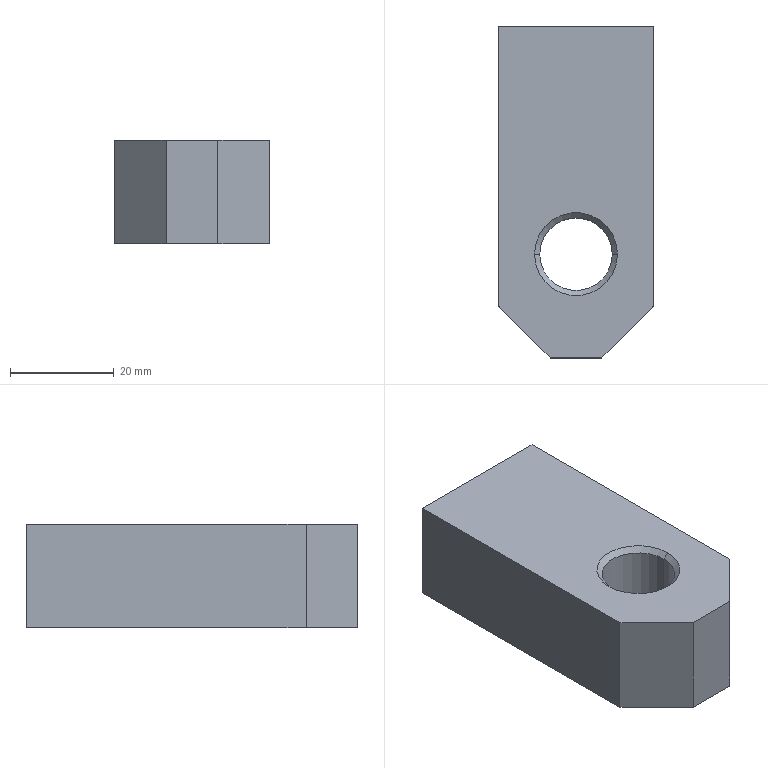Part | STEP file | BCC3 H12_4B | 1 solid | 18 faces | box 30 x 64 x 20 mm | volume 31837 mm3 | plane 8 | cone 6 | cylinder 4 | commonest cylinder face diameters 8.5 x2 14 x2
STEP:
#1=CARTESIAN_POINT('',(0.,0.,0.));
#2=DIRECTION('',(0.,0.,1.));
#3=DIRECTION('',(1.,0.,0.));
#4=AXIS2_PLACEMENT_3D('',#1,#2,#3);
#5=CARTESIAN_POINT('',(7.,-12.,9.));
#6=VERTEX_POINT('',#5);
#7=CARTESIAN_POINT('',(8.,-12.,10.));
#8=VERTEX_POINT('',#7);
#9=CARTESIAN_POINT('',(7.,-12.,9.));
#10=DIRECTION('',(0.7071,0.,0.7071));
#11=VECTOR('',#10,1.);
#12=LINE('',#9,#11);
#13=CARTESIAN_POINT('',(0.,-12.,9.));
#14=DIRECTION('',(0.,0.,1.));
#15=DIRECTION('',(1.,0.,0.));
#16=AXIS2_PLACEMENT_3D('',#13,#14,#15);
#17=CONICAL_SURFACE('',#16,7.,0.7854);
#18=CARTESIAN_POINT('',(6.283,0.));
#19=DIRECTION('',(0.,1.));
#20=VECTOR('',#19,1.);
#21=LINE('',#18,#20);
#22=(GEOMETRIC_REPRESENTATION_CONTEXT(2)PARAMETRIC_REPRESENTATION_CONTEXT()REPRESENTATION_CONTEXT('',''));
#23=DEFINITIONAL_REPRESENTATION('',(#21),#22);
#24=PCURVE('',#17,#23);
#25=CARTESIAN_POINT('',(0.,-12.,9.));
#26=DIRECTION('',(0.,0.,1.));
#27=DIRECTION('',(1.,0.,0.));
#28=AXIS2_PLACEMENT_3D('',#25,#26,#27);
#29=CONICAL_SURFACE('',#28,7.,0.7854);
#30=CARTESIAN_POINT('',(0.,0.));
#31=DIRECTION('',(0.,1.));
#32=VECTOR('',#31,1.);
#33=LINE('',#30,#32);
#34=(GEOMETRIC_REPRESENTATION_CONTEXT(2)PARAMETRIC_REPRESENTATION_CONTEXT()REPRESENTATION_CONTEXT('',''));
#35=DEFINITIONAL_REPRESENTATION('',(#33),#34);
#36=PCURVE('',#29,#35);
#37=SURFACE_CURVE('',#12,(#24,#36),.PCURVE_S1.);
#38=EDGE_CURVE('',#6,#8,#37,.T.);
#39=ORIENTED_EDGE('',*,*,#38,.T.);
#40=CARTESIAN_POINT('',(-8.,-12.,10.));
#41=VERTEX_POINT('',#40);
#42=CARTESIAN_POINT('',(0.,-12.,10.));
#43=DIRECTION('',(0.,0.,-1.));
#44=DIRECTION('',(1.,0.,0.));
#45=AXIS2_PLACEMENT_3D('',#42,#43,#44);
#46=CIRCLE('',#45,8.);
#47=CARTESIAN_POINT('',(6.283,1.));
#48=DIRECTION('',(-1.,0.));
#49=VECTOR('',#48,1.);
#50=LINE('',#47,#49);
#51=(GEOMETRIC_REPRESENTATION_CONTEXT(2)PARAMETRIC_REPRESENTATION_CONTEXT()REPRESENTATION_CONTEXT('',''));
#52=DEFINITIONAL_REPRESENTATION('',(#50),#51);
#53=PCURVE('',#17,#52);
#54=CARTESIAN_POINT('',(0.,0.,10.));
#55=DIRECTION('',(0.,0.,1.));
#56=DIRECTION('',(1.,0.,0.));
#57=AXIS2_PLACEMENT_3D('',#54,#55,#56);
#58=PLANE('',#57);
#59=CARTESIAN_POINT('',(8.,-12.));
#60=CARTESIAN_POINT('',(8.,-25.856));
#61=CARTESIAN_POINT('',(-4.,-18.928));
#62=CARTESIAN_POINT('',(-16.,-12.));
#63=CARTESIAN_POINT('',(-4.,-5.072));
#64=CARTESIAN_POINT('',(8.,1.856));
#65=CARTESIAN_POINT('',(8.,-12.));
#66=(BOUNDED_CURVE()B_SPLINE_CURVE(2,(#59,#60,#61,#62,#63,#64,#65),.UNSPECIFIED.,.T.,.F.)B_SPLINE_CURVE_WITH_KNOTS((1,2,2,2,2,1),(-2.094,0.,2.094,4.189,6.283,8.378),.UNSPECIFIED.)CURVE()GEOMETRIC_REPRESENTATION_ITEM()RATIONAL_B_SPLINE_CURVE((1.,0.5,1.,0.5,1.,0.5,1.))REPRESENTATION_ITEM(''));
#67=(GEOMETRIC_REPRESENTATION_CONTEXT(2)PARAMETRIC_REPRESENTATION_CONTEXT()REPRESENTATION_CONTEXT('',''));
#68=DEFINITIONAL_REPRESENTATION('',(#66),#67);
#69=PCURVE('',#58,#68);
#70=SURFACE_CURVE('',#46,(#53,#69),.PCURVE_S1.);
#71=EDGE_CURVE('',#8,#41,#70,.T.);
#72=ORIENTED_EDGE('',*,*,#71,.T.);
#73=CARTESIAN_POINT('',(-7.,-12.,9.));
#74=VERTEX_POINT('',#73);
#75=CARTESIAN_POINT('',(-7.,-12.,9.));
#76=DIRECTION('',(-0.7071,0.,0.7071));
#77=VECTOR('',#76,1.);
#78=LINE('',#75,#77);
#79=CARTESIAN_POINT('',(3.142,0.));
#80=DIRECTION('',(0.,1.));
#81=VECTOR('',#80,1.);
#82=LINE('',#79,#81);
#83=(GEOMETRIC_REPRESENTATION_CONTEXT(2)PARAMETRIC_REPRESENTATION_CONTEXT()REPRESENTATION_CONTEXT('',''));
#84=DEFINITIONAL_REPRESENTATION('',(#82),#83);
#85=PCURVE('',#17,#84);
#86=CARTESIAN_POINT('',(3.142,0.));
#87=DIRECTION('',(0.,1.));
#88=VECTOR('',#87,1.);
#89=LINE('',#86,#88);
#90=(GEOMETRIC_REPRESENTATION_CONTEXT(2)PARAMETRIC_REPRESENTATION_CONTEXT()REPRESENTATION_CONTEXT('',''));
#91=DEFINITIONAL_REPRESENTATION('',(#89),#90);
#92=PCURVE('',#29,#91);
#93=SURFACE_CURVE('',#78,(#85,#92),.PCURVE_S1.);
#94=EDGE_CURVE('',#74,#41,#93,.T.);
#95=ORIENTED_EDGE('',*,*,#94,.F.);
#96=CARTESIAN_POINT('',(0.,-12.,9.));
#97=DIRECTION('',(0.,0.,1.));
#98=DIRECTION('',(1.,0.,0.));
#99=AXIS2_PLACEMENT_3D('',#96,#97,#98);
#100=CIRCLE('',#99,7.);
#101=CARTESIAN_POINT('',(0.,0.));
#102=DIRECTION('',(1.,0.));
#103=VECTOR('',#102,1.);
#104=LINE('',#101,#103);
#105=(GEOMETRIC_REPRESENTATION_CONTEXT(2)PARAMETRIC_REPRESENTATION_CONTEXT()REPRESENTATION_CONTEXT('',''));
#106=DEFINITIONAL_REPRESENTATION('',(#104),#105);
#107=PCURVE('',#17,#106);
#108=CARTESIAN_POINT('',(0.,-12.,10.));
#109=DIRECTION('',(0.,0.,-1.));
#110=DIRECTION('',(-1.,0.,0.));
#111=AXIS2_PLACEMENT_3D('',#108,#109,#110);
#112=CYLINDRICAL_SURFACE('',#111,7.);
#113=CARTESIAN_POINT('',(9.425,1.));
#114=DIRECTION('',(-1.,0.));
#115=VECTOR('',#114,1.);
#116=LINE('',#113,#115);
#117=(GEOMETRIC_REPRESENTATION_CONTEXT(2)PARAMETRIC_REPRESENTATION_CONTEXT()REPRESENTATION_CONTEXT('',''));
#118=DEFINITIONAL_REPRESENTATION('',(#116),#117);
#119=PCURVE('',#112,#118);
#120=SURFACE_CURVE('',#100,(#107,#119),.PCURVE_S1.);
#121=EDGE_CURVE('',#74,#6,#120,.T.);
#122=ORIENTED_EDGE('',*,*,#121,.T.);
#123=EDGE_LOOP('',(#39,#72,#95,#122));
#124=FACE_BOUND('',#123,.F.);
#125=ADVANCED_FACE('',(#124),#17,.F.);
#126=CARTESIAN_POINT('',(-7.,-12.,-9.));
#127=VERTEX_POINT('',#126);
#128=CARTESIAN_POINT('',(-8.,-12.,-10.));
#129=VERTEX_POINT('',#128);
#130=CARTESIAN_POINT('',(-8.,-12.,-10.));
#131=DIRECTION('',(-0.7071,0.,-0.7071));
#132=VECTOR('',#131,1.);
#133=LINE('',#130,#132);
#134=CARTESIAN_POINT('',(0.,-12.,-10.));
#135=DIRECTION('',(0.,0.,-1.));
#136=DIRECTION('',(-1.,0.,0.));
#137=AXIS2_PLACEMENT_3D('',#134,#135,#136);
#138=CONICAL_SURFACE('',#137,8.,0.7854);
#139=CARTESIAN_POINT('',(6.283,0.));
#140=DIRECTION('',(0.,1.));
#141=VECTOR('',#140,1.);
#142=LINE('',#139,#141);
#143=(GEOMETRIC_REPRESENTATION_CONTEXT(2)PARAMETRIC_REPRESENTATION_CONTEXT()REPRESENTATION_CONTEXT('',''));
#144=DEFINITIONAL_REPRESENTATION('',(#142),#143);
#145=PCURVE('',#138,#144);
#146=CARTESIAN_POINT('',(0.,-12.,-10.));
#147=DIRECTION('',(0.,0.,-1.));
#148=DIRECTION('',(-1.,0.,0.));
#149=AXIS2_PLACEMENT_3D('',#146,#147,#148);
#150=CONICAL_SURFACE('',#149,8.,0.7854);
#151=CARTESIAN_POINT('',(0.,0.));
#152=DIRECTION('',(0.,1.));
#153=VECTOR('',#152,1.);
#154=LINE('',#151,#153);
#155=(GEOMETRIC_REPRESENTATION_CONTEXT(2)PARAMETRIC_REPRESENTATION_CONTEXT()REPRESENTATION_CONTEXT('',''));
#156=DEFINITIONAL_REPRESENTATION('',(#154),#155);
#157=PCURVE('',#150,#156);
#158=SURFACE_CURVE('',#133,(#145,#157),.PCURVE_S1.);
#159=EDGE_CURVE('',#127,#129,#158,.T.);
#160=ORIENTED_EDGE('',*,*,#159,.T.);
#161=CARTESIAN_POINT('',(8.,-12.,-10.));
#162=VERTEX_POINT('',#161);
#163=CARTESIAN_POINT('',(0.,-12.,-10.));
#164=DIRECTION('',(0.,0.,1.));
#165=DIRECTION('',(1.,0.,0.));
#166=AXIS2_PLACEMENT_3D('',#163,#164,#165);
#167=CIRCLE('',#166,8.);
#168=CARTESIAN_POINT('',(9.425,0.));
#169=DIRECTION('',(-1.,0.));
#170=VECTOR('',#169,1.);
#171=LINE('',#168,#170);
#172=(GEOMETRIC_REPRESENTATION_CONTEXT(2)PARAMETRIC_REPRESENTATION_CONTEXT()REPRESENTATION_CONTEXT('',''));
#173=DEFINITIONAL_REPRESENTATION('',(#171),#172);
#174=PCURVE('',#138,#173);
#175=CARTESIAN_POINT('',(0.,0.,-10.));
#176=DIRECTION('',(0.,0.,1.));
#177=DIRECTION('',(1.,0.,0.));
#178=AXIS2_PLACEMENT_3D('',#175,#176,#177);
#179=PLANE('',#178);
#180=CARTESIAN_POINT('',(0.,-12.));
#181=DIRECTION('',(1.,0.));
#182=AXIS2_PLACEMENT_2D('',#180,#181);
#183=CIRCLE('',#182,8.);
#184=(GEOMETRIC_REPRESENTATION_CONTEXT(2)PARAMETRIC_REPRESENTATION_CONTEXT()REPRESENTATION_CONTEXT('',''));
#185=DEFINITIONAL_REPRESENTATION('',(#183),#184);
#186=PCURVE('',#179,#185);
#187=SURFACE_CURVE('',#167,(#174,#186),.PCURVE_S1.);
#188=EDGE_CURVE('',#129,#162,#187,.T.);
#189=ORIENTED_EDGE('',*,*,#188,.T.);
#190=CARTESIAN_POINT('',(7.,-12.,-9.));
#191=VERTEX_POINT('',#190);
#192=CARTESIAN_POINT('',(8.,-12.,-10.));
#193=DIRECTION('',(0.7071,0.,-0.7071));
#194=VECTOR('',#193,1.);
#195=LINE('',#192,#194);
#196=CARTESIAN_POINT('',(3.142,0.));
#197=DIRECTION('',(0.,1.));
#198=VECTOR('',#197,1.);
#199=LINE('',#196,#198);
#200=(GEOMETRIC_REPRESENTATION_CONTEXT(2)PARAMETRIC_REPRESENTATION_CONTEXT()REPRESENTATION_CONTEXT('',''));
#201=DEFINITIONAL_REPRESENTATION('',(#199),#200);
#202=PCURVE('',#138,#201);
#203=CARTESIAN_POINT('',(3.142,0.));
#204=DIRECTION('',(0.,1.));
#205=VECTOR('',#204,1.);
#206=LINE('',#203,#205);
#207=(GEOMETRIC_REPRESENTATION_CONTEXT(2)PARAMETRIC_REPRESENTATION_CONTEXT()REPRESENTATION_CONTEXT('',''));
#208=DEFINITIONAL_REPRESENTATION('',(#206),#207);
#209=PCURVE('',#150,#208);
#210=SURFACE_CURVE('',#195,(#202,#209),.PCURVE_S1.);
#211=EDGE_CURVE('',#191,#162,#210,.T.);
#212=ORIENTED_EDGE('',*,*,#211,.F.);
#213=CARTESIAN_POINT('',(0.,-12.,-9.));
#214=DIRECTION('',(0.,0.,-1.));
#215=DIRECTION('',(1.,0.,0.));
#216=AXIS2_PLACEMENT_3D('',#213,#214,#215);
#217=CIRCLE('',#216,7.);
#218=CARTESIAN_POINT('',(3.142,-1.));
#219=DIRECTION('',(1.,0.));
#220=VECTOR('',#219,1.);
#221=LINE('',#218,#220);
#222=(GEOMETRIC_REPRESENTATION_CONTEXT(2)PARAMETRIC_REPRESENTATION_CONTEXT()REPRESENTATION_CONTEXT('',''));
#223=DEFINITIONAL_REPRESENTATION('',(#221),#222);
#224=PCURVE('',#138,#223);
#225=CARTESIAN_POINT('',(3.142,19.));
#226=DIRECTION('',(1.,0.));
#227=VECTOR('',#226,1.);
#228=LINE('',#225,#227);
#229=(GEOMETRIC_REPRESENTATION_CONTEXT(2)PARAMETRIC_REPRESENTATION_CONTEXT()REPRESENTATION_CONTEXT('',''));
#230=DEFINITIONAL_REPRESENTATION('',(#228),#229);
#231=PCURVE('',#112,#230);
#232=SURFACE_CURVE('',#217,(#224,#231),.PCURVE_S1.);
#233=EDGE_CURVE('',#191,#127,#232,.T.);
#234=ORIENTED_EDGE('',*,*,#233,.T.);
#235=EDGE_LOOP('',(#160,#189,#212,#234));
#236=FACE_BOUND('',#235,.F.);
#237=ADVANCED_FACE('',(#236),#138,.F.);
#238=CARTESIAN_POINT('',(0.,7.5,4.25));
#239=VERTEX_POINT('',#238);
#240=CARTESIAN_POINT('',(0.,32.,4.25));
#241=VERTEX_POINT('',#240);
#242=CARTESIAN_POINT('',(0.,32.,4.25));
#243=DIRECTION('',(0.,1.,0.));
#244=VECTOR('',#243,1.);
#245=LINE('',#242,#244);
#246=CARTESIAN_POINT('',(0.,32.,0.));
#247=DIRECTION('',(0.,1.,0.));
#248=DIRECTION('',(0.,0.,1.));
#249=AXIS2_PLACEMENT_3D('',#246,#247,#248);
#250=CYLINDRICAL_SURFACE('',#249,4.25);
#251=CARTESIAN_POINT('',(6.283,0.));
#252=DIRECTION('',(0.,1.));
#253=VECTOR('',#252,1.);
#254=LINE('',#251,#253);
#255=(GEOMETRIC_REPRESENTATION_CONTEXT(2)PARAMETRIC_REPRESENTATION_CONTEXT()REPRESENTATION_CONTEXT('',''));
#256=DEFINITIONAL_REPRESENTATION('',(#254),#255);
#257=PCURVE('',#250,#256);
#258=CARTESIAN_POINT('',(0.,32.,0.));
#259=DIRECTION('',(0.,1.,0.));
#260=DIRECTION('',(0.,0.,1.));
#261=AXIS2_PLACEMENT_3D('',#258,#259,#260);
#262=CYLINDRICAL_SURFACE('',#261,4.25);
#263=CARTESIAN_POINT('',(0.,0.));
#264=DIRECTION('',(0.,1.));
#265=VECTOR('',#264,1.);
#266=LINE('',#263,#265);
#267=(GEOMETRIC_REPRESENTATION_CONTEXT(2)PARAMETRIC_REPRESENTATION_CONTEXT()REPRESENTATION_CONTEXT('',''));
#268=DEFINITIONAL_REPRESENTATION('',(#266),#267);
#269=PCURVE('',#262,#268);
#270=SURFACE_CURVE('',#245,(#257,#269),.PCURVE_S1.);
#271=EDGE_CURVE('',#239,#241,#270,.T.);
#272=ORIENTED_EDGE('',*,*,#271,.T.);
#273=CARTESIAN_POINT('',(0.,32.,-4.25));
#274=VERTEX_POINT('',#273);
#275=CARTESIAN_POINT('',(0.,32.,0.));
#276=DIRECTION('',(0.,1.,0.));
#277=DIRECTION('',(0.,0.,1.));
#278=AXIS2_PLACEMENT_3D('',#275,#276,#277);
#279=CIRCLE('',#278,4.25);
#280=CARTESIAN_POINT('',(0.,0.));
#281=DIRECTION('',(1.,0.));
#282=VECTOR('',#281,1.);
#283=LINE('',#280,#282);
#284=(GEOMETRIC_REPRESENTATION_CONTEXT(2)PARAMETRIC_REPRESENTATION_CONTEXT()REPRESENTATION_CONTEXT('',''));
#285=DEFINITIONAL_REPRESENTATION('',(#283),#284);
#286=PCURVE('',#250,#285);
#287=CARTESIAN_POINT('',(-15.,32.,10.));
#288=DIRECTION('',(0.,-1.,0.));
#289=DIRECTION('',(0.,0.,-1.));
#290=AXIS2_PLACEMENT_3D('',#287,#288,#289);
#291=PLANE('',#290);
#292=CARTESIAN_POINT('',(5.75,15.));
#293=CARTESIAN_POINT('',(5.75,22.361));
#294=CARTESIAN_POINT('',(12.125,18.681));
#295=CARTESIAN_POINT('',(18.5,15.));
#296=CARTESIAN_POINT('',(12.125,11.319));
#297=CARTESIAN_POINT('',(5.75,7.639));
#298=CARTESIAN_POINT('',(5.75,15.));
#299=(BOUNDED_CURVE()B_SPLINE_CURVE(2,(#292,#293,#294,#295,#296,#297,#298),.UNSPECIFIED.,.T.,.F.)B_SPLINE_CURVE_WITH_KNOTS((1,2,2,2,2,1),(-2.094,0.,2.094,4.189,6.283,8.378),.UNSPECIFIED.)CURVE()GEOMETRIC_REPRESENTATION_ITEM()RATIONAL_B_SPLINE_CURVE((1.,0.5,1.,0.5,1.,0.5,1.))REPRESENTATION_ITEM(''));
#300=(GEOMETRIC_REPRESENTATION_CONTEXT(2)PARAMETRIC_REPRESENTATION_CONTEXT()REPRESENTATION_CONTEXT('',''));
#301=DEFINITIONAL_REPRESENTATION('',(#299),#300);
#302=PCURVE('',#291,#301);
#303=SURFACE_CURVE('',#279,(#286,#302),.PCURVE_S1.);
#304=EDGE_CURVE('',#274,#241,#303,.T.);
#305=ORIENTED_EDGE('',*,*,#304,.F.);
#306=CARTESIAN_POINT('',(0.,7.5,-4.25));
#307=VERTEX_POINT('',#306);
#308=CARTESIAN_POINT('',(0.,32.,-4.25));
#309=DIRECTION('',(0.,1.,0.));
#310=VECTOR('',#309,1.);
#311=LINE('',#308,#310);
#312=CARTESIAN_POINT('',(3.142,0.));
#313=DIRECTION('',(0.,1.));
#314=VECTOR('',#313,1.);
#315=LINE('',#312,#314);
#316=(GEOMETRIC_REPRESENTATION_CONTEXT(2)PARAMETRIC_REPRESENTATION_CONTEXT()REPRESENTATION_CONTEXT('',''));
#317=DEFINITIONAL_REPRESENTATION('',(#315),#316);
#318=PCURVE('',#250,#317);
#319=CARTESIAN_POINT('',(3.142,0.));
#320=DIRECTION('',(0.,1.));
#321=VECTOR('',#320,1.);
#322=LINE('',#319,#321);
#323=(GEOMETRIC_REPRESENTATION_CONTEXT(2)PARAMETRIC_REPRESENTATION_CONTEXT()REPRESENTATION_CONTEXT('',''));
#324=DEFINITIONAL_REPRESENTATION('',(#322),#323);
#325=PCURVE('',#262,#324);
#326=SURFACE_CURVE('',#311,(#318,#325),.PCURVE_S1.);
#327=EDGE_CURVE('',#307,#274,#326,.T.);
#328=ORIENTED_EDGE('',*,*,#327,.F.);
#329=CARTESIAN_POINT('',(0.,7.5,0.));
#330=DIRECTION('',(0.,1.,0.));
#331=DIRECTION('',(0.,0.,1.));
#332=AXIS2_PLACEMENT_3D('',#329,#330,#331);
#333=CIRCLE('',#332,4.25);
#334=CARTESIAN_POINT('',(0.,-24.5));
#335=DIRECTION('',(1.,0.));
#336=VECTOR('',#335,1.);
#337=LINE('',#334,#336);
#338=(GEOMETRIC_REPRESENTATION_CONTEXT(2)PARAMETRIC_REPRESENTATION_CONTEXT()REPRESENTATION_CONTEXT('',''));
#339=DEFINITIONAL_REPRESENTATION('',(#337),#338);
#340=PCURVE('',#250,#339);
#341=CARTESIAN_POINT('',(0.,7.5,0.));
#342=DIRECTION('',(0.,1.,0.));
#343=DIRECTION('',(0.,0.,1.));
#344=AXIS2_PLACEMENT_3D('',#341,#342,#343);
#345=CONICAL_SURFACE('',#344,4.25,1.03);
#346=CARTESIAN_POINT('',(0.,0.));
#347=DIRECTION('',(1.,0.));
#348=VECTOR('',#347,1.);
#349=LINE('',#346,#348);
#350=(GEOMETRIC_REPRESENTATION_CONTEXT(2)PARAMETRIC_REPRESENTATION_CONTEXT()REPRESENTATION_CONTEXT('',''));
#351=DEFINITIONAL_REPRESENTATION('',(#349),#350);
#352=PCURVE('',#345,#351);
#353=SURFACE_CURVE('',#333,(#340,#352),.PCURVE_S1.);
#354=EDGE_CURVE('',#307,#239,#353,.T.);
#355=ORIENTED_EDGE('',*,*,#354,.T.);
#356=EDGE_LOOP('',(#272,#305,#328,#355));
#357=FACE_BOUND('',#356,.F.);
#358=ADVANCED_FACE('',(#357),#250,.F.);
#359=ORIENTED_EDGE('',*,*,#354,.F.);
#360=CARTESIAN_POINT('',(0.,4.946,0.));
#361=VERTEX_POINT('',#360);
#362=CARTESIAN_POINT('',(0.,7.5,-4.25));
#363=DIRECTION('',(0.,0.515,-0.8572));
#364=VECTOR('',#363,1.);
#365=LINE('',#362,#364);
#366=CARTESIAN_POINT('',(3.142,0.));
#367=DIRECTION('',(0.,1.));
#368=VECTOR('',#367,1.);
#369=LINE('',#366,#368);
#370=(GEOMETRIC_REPRESENTATION_CONTEXT(2)PARAMETRIC_REPRESENTATION_CONTEXT()REPRESENTATION_CONTEXT('',''));
#371=DEFINITIONAL_REPRESENTATION('',(#369),#370);
#372=PCURVE('',#345,#371);
#373=CARTESIAN_POINT('',(0.,7.5,0.));
#374=DIRECTION('',(0.,1.,0.));
#375=DIRECTION('',(0.,0.,1.));
#376=AXIS2_PLACEMENT_3D('',#373,#374,#375);
#377=CONICAL_SURFACE('',#376,4.25,1.03);
#378=CARTESIAN_POINT('',(3.142,0.));
#379=DIRECTION('',(0.,1.));
#380=VECTOR('',#379,1.);
#381=LINE('',#378,#380);
#382=(GEOMETRIC_REPRESENTATION_CONTEXT(2)PARAMETRIC_REPRESENTATION_CONTEXT()REPRESENTATION_CONTEXT('',''));
#383=DEFINITIONAL_REPRESENTATION('',(#381),#382);
#384=PCURVE('',#377,#383);
#385=SURFACE_CURVE('',#365,(#372,#384),.PCURVE_S1.);
#386=EDGE_CURVE('',#361,#307,#385,.T.);
#387=ORIENTED_EDGE('',*,*,#386,.F.);
#388=CARTESIAN_POINT('',(0.,7.5,4.25));
#389=DIRECTION('',(0.,0.515,0.8572));
#390=VECTOR('',#389,1.);
#391=LINE('',#388,#390);
#392=CARTESIAN_POINT('',(6.283,0.));
#393=DIRECTION('',(0.,1.));
#394=VECTOR('',#393,1.);
#395=LINE('',#392,#394);
#396=(GEOMETRIC_REPRESENTATION_CONTEXT(2)PARAMETRIC_REPRESENTATION_CONTEXT()REPRESENTATION_CONTEXT('',''));
#397=DEFINITIONAL_REPRESENTATION('',(#395),#396);
#398=PCURVE('',#345,#397);
#399=CARTESIAN_POINT('',(0.,0.));
#400=DIRECTION('',(0.,1.));
#401=VECTOR('',#400,1.);
#402=LINE('',#399,#401);
#403=(GEOMETRIC_REPRESENTATION_CONTEXT(2)PARAMETRIC_REPRESENTATION_CONTEXT()REPRESENTATION_CONTEXT('',''));
#404=DEFINITIONAL_REPRESENTATION('',(#402),#403);
#405=PCURVE('',#377,#404);
#406=SURFACE_CURVE('',#391,(#398,#405),.PCURVE_S1.);
#407=EDGE_CURVE('',#361,#239,#406,.T.);
#408=ORIENTED_EDGE('',*,*,#407,.T.);
#409=EDGE_LOOP('',(#359,#387,#408));
#410=FACE_BOUND('',#409,.F.);
#411=ADVANCED_FACE('',(#410),#345,.F.);
#412=CARTESIAN_POINT('',(-7.,-12.,10.));
#413=DIRECTION('',(0.,0.,-1.));
#414=VECTOR('',#413,1.);
#415=LINE('',#412,#414);
#416=CARTESIAN_POINT('',(6.283,0.));
#417=DIRECTION('',(0.,1.));
#418=VECTOR('',#417,1.);
#419=LINE('',#416,#418);
#420=(GEOMETRIC_REPRESENTATION_CONTEXT(2)PARAMETRIC_REPRESENTATION_CONTEXT()REPRESENTATION_CONTEXT('',''));
#421=DEFINITIONAL_REPRESENTATION('',(#419),#420);
#422=PCURVE('',#112,#421);
#423=CARTESIAN_POINT('',(0.,-12.,10.));
#424=DIRECTION('',(0.,0.,-1.));
#425=DIRECTION('',(-1.,0.,0.));
#426=AXIS2_PLACEMENT_3D('',#423,#424,#425);
#427=CYLINDRICAL_SURFACE('',#426,7.);
#428=CARTESIAN_POINT('',(0.,0.));
#429=DIRECTION('',(0.,1.));
#430=VECTOR('',#429,1.);
#431=LINE('',#428,#430);
#432=(GEOMETRIC_REPRESENTATION_CONTEXT(2)PARAMETRIC_REPRESENTATION_CONTEXT()REPRESENTATION_CONTEXT('',''));
#433=DEFINITIONAL_REPRESENTATION('',(#431),#432);
#434=PCURVE('',#427,#433);
#435=SURFACE_CURVE('',#415,(#422,#434),.PCURVE_S1.);
#436=EDGE_CURVE('',#74,#127,#435,.T.);
#437=ORIENTED_EDGE('',*,*,#436,.T.);
#438=ORIENTED_EDGE('',*,*,#233,.F.);
#439=CARTESIAN_POINT('',(7.,-12.,10.));
#440=DIRECTION('',(0.,0.,-1.));
#441=VECTOR('',#440,1.);
#442=LINE('',#439,#441);
#443=CARTESIAN_POINT('',(3.142,0.));
#444=DIRECTION('',(0.,1.));
#445=VECTOR('',#444,1.);
#446=LINE('',#443,#445);
#447=(GEOMETRIC_REPRESENTATION_CONTEXT(2)PARAMETRIC_REPRESENTATION_CONTEXT()REPRESENTATION_CONTEXT('',''));
#448=DEFINITIONAL_REPRESENTATION('',(#446),#447);
#449=PCURVE('',#112,#448);
#450=CARTESIAN_POINT('',(3.142,0.));
#451=DIRECTION('',(0.,1.));
#452=VECTOR('',#451,1.);
#453=LINE('',#450,#452);
#454=(GEOMETRIC_REPRESENTATION_CONTEXT(2)PARAMETRIC_REPRESENTATION_CONTEXT()REPRESENTATION_CONTEXT('',''));
#455=DEFINITIONAL_REPRESENTATION('',(#453),#454);
#456=PCURVE('',#427,#455);
#457=SURFACE_CURVE('',#442,(#449,#456),.PCURVE_S1.);
#458=EDGE_CURVE('',#6,#191,#457,.T.);
#459=ORIENTED_EDGE('',*,*,#458,.F.);
#460=ORIENTED_EDGE('',*,*,#121,.F.);
#461=EDGE_LOOP('',(#437,#438,#459,#460));
#462=FACE_BOUND('',#461,.F.);
#463=ADVANCED_FACE('',(#462),#112,.F.);
#464=ORIENTED_EDGE('',*,*,#71,.T.);
#465=CARTESIAN_POINT('',(0.,-12.,10.));
#466=DIRECTION('',(0.,0.,-1.));
#467=DIRECTION('',(1.,0.,0.));
#468=AXIS2_PLACEMENT_3D('',#465,#466,#467);
#469=CIRCLE('',#468,8.);
#470=CARTESIAN_POINT('',(8.,-12.));
#471=CARTESIAN_POINT('',(8.,-25.856));
#472=CARTESIAN_POINT('',(-4.,-18.928));
#473=CARTESIAN_POINT('',(-16.,-12.));
#474=CARTESIAN_POINT('',(-4.,-5.072));
#475=CARTESIAN_POINT('',(8.,1.856));
#476=CARTESIAN_POINT('',(8.,-12.));
#477=(BOUNDED_CURVE()B_SPLINE_CURVE(2,(#470,#471,#472,#473,#474,#475,#476),.UNSPECIFIED.,.T.,.F.)B_SPLINE_CURVE_WITH_KNOTS((1,2,2,2,2,1),(-2.094,0.,2.094,4.189,6.283,8.378),.UNSPECIFIED.)CURVE()GEOMETRIC_REPRESENTATION_ITEM()RATIONAL_B_SPLINE_CURVE((1.,0.5,1.,0.5,1.,0.5,1.))REPRESENTATION_ITEM(''));
#478=(GEOMETRIC_REPRESENTATION_CONTEXT(2)PARAMETRIC_REPRESENTATION_CONTEXT()REPRESENTATION_CONTEXT('',''));
#479=DEFINITIONAL_REPRESENTATION('',(#477),#478);
#480=PCURVE('',#58,#479);
#481=CARTESIAN_POINT('',(6.283,1.));
#482=DIRECTION('',(-1.,0.));
#483=VECTOR('',#482,1.);
#484=LINE('',#481,#483);
#485=(GEOMETRIC_REPRESENTATION_CONTEXT(2)PARAMETRIC_REPRESENTATION_CONTEXT()REPRESENTATION_CONTEXT('',''));
#486=DEFINITIONAL_REPRESENTATION('',(#484),#485);
#487=PCURVE('',#29,#486);
#488=SURFACE_CURVE('',#469,(#480,#487),.PCURVE_S1.);
#489=EDGE_CURVE('',#41,#8,#488,.T.);
#490=ORIENTED_EDGE('',*,*,#489,.T.);
#491=EDGE_LOOP('',(#464,#490));
#492=FACE_BOUND('',#491,.T.);
#493=CARTESIAN_POINT('',(-15.,32.,10.));
#494=VERTEX_POINT('',#493);
#495=CARTESIAN_POINT('',(-15.,-22.,10.));
#496=VERTEX_POINT('',#495);
#497=CARTESIAN_POINT('',(-15.,32.,10.));
#498=DIRECTION('',(0.,-1.,0.));
#499=VECTOR('',#498,1.);
#500=LINE('',#497,#499);
#501=CARTESIAN_POINT('',(-15.,32.));
#502=DIRECTION('',(0.,-1.));
#503=VECTOR('',#502,1.);
#504=LINE('',#501,#503);
#505=(GEOMETRIC_REPRESENTATION_CONTEXT(2)PARAMETRIC_REPRESENTATION_CONTEXT()REPRESENTATION_CONTEXT('',''));
#506=DEFINITIONAL_REPRESENTATION('',(#504),#505);
#507=PCURVE('',#58,#506);
#508=CARTESIAN_POINT('',(-15.,32.,10.));
#509=DIRECTION('',(1.,0.,0.));
#510=DIRECTION('',(0.,1.,0.));
#511=AXIS2_PLACEMENT_3D('',#508,#509,#510);
#512=PLANE('',#511);
#513=CARTESIAN_POINT('',(0.,0.));
#514=DIRECTION('',(-1.,0.));
#515=VECTOR('',#514,1.);
#516=LINE('',#513,#515);
#517=(GEOMETRIC_REPRESENTATION_CONTEXT(2)PARAMETRIC_REPRESENTATION_CONTEXT()REPRESENTATION_CONTEXT('',''));
#518=DEFINITIONAL_REPRESENTATION('',(#516),#517);
#519=PCURVE('',#512,#518);
#520=SURFACE_CURVE('',#500,(#507,#519),.PCURVE_S1.);
#521=EDGE_CURVE('',#494,#496,#520,.T.);
#522=ORIENTED_EDGE('',*,*,#521,.T.);
#523=CARTESIAN_POINT('',(-5.,-32.,10.));
#524=VERTEX_POINT('',#523);
#525=CARTESIAN_POINT('',(-18.5,-18.5,10.));
#526=DIRECTION('',(0.7071,-0.7071,0.));
#527=VECTOR('',#526,1.);
#528=LINE('',#525,#527);
#529=CARTESIAN_POINT('',(-18.5,-18.5));
#530=DIRECTION('',(0.7071,-0.7071));
#531=VECTOR('',#530,1.);
#532=LINE('',#529,#531);
#533=(GEOMETRIC_REPRESENTATION_CONTEXT(2)PARAMETRIC_REPRESENTATION_CONTEXT()REPRESENTATION_CONTEXT('',''));
#534=DEFINITIONAL_REPRESENTATION('',(#532),#533);
#535=PCURVE('',#58,#534);
#536=CARTESIAN_POINT('',(-5.,-32.,10.));
#537=DIRECTION('',(0.7071,0.7071,0.));
#538=DIRECTION('',(0.,0.,-1.));
#539=AXIS2_PLACEMENT_3D('',#536,#537,#538);
#540=PLANE('',#539);
#541=CARTESIAN_POINT('',(0.,19.092));
#542=DIRECTION('',(0.,-1.));
#543=VECTOR('',#542,1.);
#544=LINE('',#541,#543);
#545=(GEOMETRIC_REPRESENTATION_CONTEXT(2)PARAMETRIC_REPRESENTATION_CONTEXT()REPRESENTATION_CONTEXT('',''));
#546=DEFINITIONAL_REPRESENTATION('',(#544),#545);
#547=PCURVE('',#540,#546);
#548=SURFACE_CURVE('',#528,(#535,#547),.PCURVE_S1.);
#549=EDGE_CURVE('',#496,#524,#548,.T.);
#550=ORIENTED_EDGE('',*,*,#549,.T.);
#551=CARTESIAN_POINT('',(5.,-32.,10.));
#552=VERTEX_POINT('',#551);
#553=CARTESIAN_POINT('',(-15.,-32.,10.));
#554=DIRECTION('',(1.,0.,0.));
#555=VECTOR('',#554,1.);
#556=LINE('',#553,#555);
#557=CARTESIAN_POINT('',(-15.,-32.));
#558=DIRECTION('',(1.,0.));
#559=VECTOR('',#558,1.);
#560=LINE('',#557,#559);
#561=(GEOMETRIC_REPRESENTATION_CONTEXT(2)PARAMETRIC_REPRESENTATION_CONTEXT()REPRESENTATION_CONTEXT('',''));
#562=DEFINITIONAL_REPRESENTATION('',(#560),#561);
#563=PCURVE('',#58,#562);
#564=CARTESIAN_POINT('',(-15.,-32.,10.));
#565=DIRECTION('',(0.,1.,0.));
#566=DIRECTION('',(0.,0.,1.));
#567=AXIS2_PLACEMENT_3D('',#564,#565,#566);
#568=PLANE('',#567);
#569=CARTESIAN_POINT('',(0.,0.));
#570=DIRECTION('',(0.,1.));
#571=VECTOR('',#570,1.);
#572=LINE('',#569,#571);
#573=(GEOMETRIC_REPRESENTATION_CONTEXT(2)PARAMETRIC_REPRESENTATION_CONTEXT()REPRESENTATION_CONTEXT('',''));
#574=DEFINITIONAL_REPRESENTATION('',(#572),#573);
#575=PCURVE('',#568,#574);
#576=SURFACE_CURVE('',#556,(#563,#575),.PCURVE_S1.);
#577=EDGE_CURVE('',#524,#552,#576,.T.);
#578=ORIENTED_EDGE('',*,*,#577,.T.);
#579=CARTESIAN_POINT('',(15.,-22.,10.));
#580=VERTEX_POINT('',#579);
#581=CARTESIAN_POINT('',(18.5,-18.5,10.));
#582=DIRECTION('',(0.7071,0.7071,0.));
#583=VECTOR('',#582,1.);
#584=LINE('',#581,#583);
#585=CARTESIAN_POINT('',(18.5,-18.5));
#586=DIRECTION('',(0.7071,0.7071));
#587=VECTOR('',#586,1.);
#588=LINE('',#585,#587);
#589=(GEOMETRIC_REPRESENTATION_CONTEXT(2)PARAMETRIC_REPRESENTATION_CONTEXT()REPRESENTATION_CONTEXT('',''));
#590=DEFINITIONAL_REPRESENTATION('',(#588),#589);
#591=PCURVE('',#58,#590);
#592=CARTESIAN_POINT('',(15.,-22.,10.));
#593=DIRECTION('',(-0.7071,0.7071,0.));
#594=DIRECTION('',(0.,0.,-1.));
#595=AXIS2_PLACEMENT_3D('',#592,#593,#594);
#596=PLANE('',#595);
#597=CARTESIAN_POINT('',(0.,-4.95));
#598=DIRECTION('',(0.,-1.));
#599=VECTOR('',#598,1.);
#600=LINE('',#597,#599);
#601=(GEOMETRIC_REPRESENTATION_CONTEXT(2)PARAMETRIC_REPRESENTATION_CONTEXT()REPRESENTATION_CONTEXT('',''));
#602=DEFINITIONAL_REPRESENTATION('',(#600),#601);
#603=PCURVE('',#596,#602);
#604=SURFACE_CURVE('',#584,(#591,#603),.PCURVE_S1.);
#605=EDGE_CURVE('',#552,#580,#604,.T.);
#606=ORIENTED_EDGE('',*,*,#605,.T.);
#607=CARTESIAN_POINT('',(15.,32.,10.));
#608=VERTEX_POINT('',#607);
#609=CARTESIAN_POINT('',(15.,32.,10.));
#610=DIRECTION('',(0.,1.,0.));
#611=VECTOR('',#610,1.);
#612=LINE('',#609,#611);
#613=CARTESIAN_POINT('',(15.,32.));
#614=DIRECTION('',(0.,1.));
#615=VECTOR('',#614,1.);
#616=LINE('',#613,#615);
#617=(GEOMETRIC_REPRESENTATION_CONTEXT(2)PARAMETRIC_REPRESENTATION_CONTEXT()REPRESENTATION_CONTEXT('',''));
#618=DEFINITIONAL_REPRESENTATION('',(#616),#617);
#619=PCURVE('',#58,#618);
#620=CARTESIAN_POINT('',(15.,32.,10.));
#621=DIRECTION('',(-1.,0.,0.));
#622=DIRECTION('',(0.,-1.,0.));
#623=AXIS2_PLACEMENT_3D('',#620,#621,#622);
#624=PLANE('',#623);
#625=CARTESIAN_POINT('',(0.,0.));
#626=DIRECTION('',(-1.,0.));
#627=VECTOR('',#626,1.);
#628=LINE('',#625,#627);
#629=(GEOMETRIC_REPRESENTATION_CONTEXT(2)PARAMETRIC_REPRESENTATION_CONTEXT()REPRESENTATION_CONTEXT('',''));
#630=DEFINITIONAL_REPRESENTATION('',(#628),#629);
#631=PCURVE('',#624,#630);
#632=SURFACE_CURVE('',#612,(#619,#631),.PCURVE_S1.);
#633=EDGE_CURVE('',#580,#608,#632,.T.);
#634=ORIENTED_EDGE('',*,*,#633,.T.);
#635=CARTESIAN_POINT('',(-15.,32.,10.));
#636=DIRECTION('',(-1.,0.,0.));
#637=VECTOR('',#636,1.);
#638=LINE('',#635,#637);
#639=CARTESIAN_POINT('',(-15.,32.));
#640=DIRECTION('',(-1.,0.));
#641=VECTOR('',#640,1.);
#642=LINE('',#639,#641);
#643=(GEOMETRIC_REPRESENTATION_CONTEXT(2)PARAMETRIC_REPRESENTATION_CONTEXT()REPRESENTATION_CONTEXT('',''));
#644=DEFINITIONAL_REPRESENTATION('',(#642),#643);
#645=PCURVE('',#58,#644);
#646=CARTESIAN_POINT('',(0.,0.));
#647=DIRECTION('',(0.,-1.));
#648=VECTOR('',#647,1.);
#649=LINE('',#646,#648);
#650=(GEOMETRIC_REPRESENTATION_CONTEXT(2)PARAMETRIC_REPRESENTATION_CONTEXT()REPRESENTATION_CONTEXT('',''));
#651=DEFINITIONAL_REPRESENTATION('',(#649),#650);
#652=PCURVE('',#291,#651);
#653=SURFACE_CURVE('',#638,(#645,#652),.PCURVE_S1.);
#654=EDGE_CURVE('',#608,#494,#653,.T.);
#655=ORIENTED_EDGE('',*,*,#654,.T.);
#656=EDGE_LOOP('',(#522,#550,#578,#606,#634,#655));
#657=FACE_BOUND('',#656,.T.);
#658=ADVANCED_FACE('',(#492,#657),#58,.T.);
#659=ORIENTED_EDGE('',*,*,#188,.T.);
#660=CARTESIAN_POINT('',(0.,-12.,-10.));
#661=DIRECTION('',(0.,0.,1.));
#662=DIRECTION('',(1.,0.,0.));
#663=AXIS2_PLACEMENT_3D('',#660,#661,#662);
#664=CIRCLE('',#663,8.);
#665=CARTESIAN_POINT('',(0.,-12.));
#666=DIRECTION('',(1.,0.));
#667=AXIS2_PLACEMENT_2D('',#665,#666);
#668=CIRCLE('',#667,8.);
#669=(GEOMETRIC_REPRESENTATION_CONTEXT(2)PARAMETRIC_REPRESENTATION_CONTEXT()REPRESENTATION_CONTEXT('',''));
#670=DEFINITIONAL_REPRESENTATION('',(#668),#669);
#671=PCURVE('',#179,#670);
#672=CARTESIAN_POINT('',(3.142,0.));
#673=DIRECTION('',(-1.,0.));
#674=VECTOR('',#673,1.);
#675=LINE('',#672,#674);
#676=(GEOMETRIC_REPRESENTATION_CONTEXT(2)PARAMETRIC_REPRESENTATION_CONTEXT()REPRESENTATION_CONTEXT('',''));
#677=DEFINITIONAL_REPRESENTATION('',(#675),#676);
#678=PCURVE('',#150,#677);
#679=SURFACE_CURVE('',#664,(#671,#678),.PCURVE_S1.);
#680=EDGE_CURVE('',#162,#129,#679,.T.);
#681=ORIENTED_EDGE('',*,*,#680,.T.);
#682=EDGE_LOOP('',(#659,#681));
#683=FACE_BOUND('',#682,.T.);
#684=CARTESIAN_POINT('',(-5.,-32.,-10.));
#685=VERTEX_POINT('',#684);
#686=CARTESIAN_POINT('',(5.,-32.,-10.));
#687=VERTEX_POINT('',#686);
#688=CARTESIAN_POINT('',(-15.,-32.,-10.));
#689=DIRECTION('',(1.,0.,0.));
#690=VECTOR('',#689,1.);
#691=LINE('',#688,#690);
#692=CARTESIAN_POINT('',(-15.,-32.));
#693=DIRECTION('',(1.,0.));
#694=VECTOR('',#693,1.);
#695=LINE('',#692,#694);
#696=(GEOMETRIC_REPRESENTATION_CONTEXT(2)PARAMETRIC_REPRESENTATION_CONTEXT()REPRESENTATION_CONTEXT('',''));
#697=DEFINITIONAL_REPRESENTATION('',(#695),#696);
#698=PCURVE('',#179,#697);
#699=CARTESIAN_POINT('',(-20.,0.));
#700=DIRECTION('',(0.,1.));
#701=VECTOR('',#700,1.);
#702=LINE('',#699,#701);
#703=(GEOMETRIC_REPRESENTATION_CONTEXT(2)PARAMETRIC_REPRESENTATION_CONTEXT()REPRESENTATION_CONTEXT('',''));
#704=DEFINITIONAL_REPRESENTATION('',(#702),#703);
#705=PCURVE('',#568,#704);
#706=SURFACE_CURVE('',#691,(#698,#705),.PCURVE_S1.);
#707=EDGE_CURVE('',#685,#687,#706,.T.);
#708=ORIENTED_EDGE('',*,*,#707,.F.);
#709=CARTESIAN_POINT('',(-15.,-22.,-10.));
#710=VERTEX_POINT('',#709);
#711=CARTESIAN_POINT('',(-5.,-32.,-10.));
#712=DIRECTION('',(-0.7071,0.7071,0.));
#713=VECTOR('',#712,1.);
#714=LINE('',#711,#713);
#715=CARTESIAN_POINT('',(-5.,-32.));
#716=DIRECTION('',(-0.7071,0.7071));
#717=VECTOR('',#716,1.);
#718=LINE('',#715,#717);
#719=(GEOMETRIC_REPRESENTATION_CONTEXT(2)PARAMETRIC_REPRESENTATION_CONTEXT()REPRESENTATION_CONTEXT('',''));
#720=DEFINITIONAL_REPRESENTATION('',(#718),#719);
#721=PCURVE('',#179,#720);
#722=CARTESIAN_POINT('',(20.,0.));
#723=DIRECTION('',(0.,1.));
#724=VECTOR('',#723,1.);
#725=LINE('',#722,#724);
#726=(GEOMETRIC_REPRESENTATION_CONTEXT(2)PARAMETRIC_REPRESENTATION_CONTEXT()REPRESENTATION_CONTEXT('',''));
#727=DEFINITIONAL_REPRESENTATION('',(#725),#726);
#728=PCURVE('',#540,#727);
#729=SURFACE_CURVE('',#714,(#721,#728),.PCURVE_S1.);
#730=EDGE_CURVE('',#685,#710,#729,.T.);
#731=ORIENTED_EDGE('',*,*,#730,.T.);
#732=CARTESIAN_POINT('',(-15.,32.,-10.));
#733=VERTEX_POINT('',#732);
#734=CARTESIAN_POINT('',(-15.,32.,-10.));
#735=DIRECTION('',(0.,-1.,0.));
#736=VECTOR('',#735,1.);
#737=LINE('',#734,#736);
#738=CARTESIAN_POINT('',(-15.,32.));
#739=DIRECTION('',(0.,-1.));
#740=VECTOR('',#739,1.);
#741=LINE('',#738,#740);
#742=(GEOMETRIC_REPRESENTATION_CONTEXT(2)PARAMETRIC_REPRESENTATION_CONTEXT()REPRESENTATION_CONTEXT('',''));
#743=DEFINITIONAL_REPRESENTATION('',(#741),#742);
#744=PCURVE('',#179,#743);
#745=CARTESIAN_POINT('',(0.,-20.));
#746=DIRECTION('',(-1.,0.));
#747=VECTOR('',#746,1.);
#748=LINE('',#745,#747);
#749=(GEOMETRIC_REPRESENTATION_CONTEXT(2)PARAMETRIC_REPRESENTATION_CONTEXT()REPRESENTATION_CONTEXT('',''));
#750=DEFINITIONAL_REPRESENTATION('',(#748),#749);
#751=PCURVE('',#512,#750);
#752=SURFACE_CURVE('',#737,(#744,#751),.PCURVE_S1.);
#753=EDGE_CURVE('',#733,#710,#752,.T.);
#754=ORIENTED_EDGE('',*,*,#753,.F.);
#755=CARTESIAN_POINT('',(15.,32.,-10.));
#756=VERTEX_POINT('',#755);
#757=CARTESIAN_POINT('',(-15.,32.,-10.));
#758=DIRECTION('',(-1.,0.,0.));
#759=VECTOR('',#758,1.);
#760=LINE('',#757,#759);
#761=CARTESIAN_POINT('',(-15.,32.));
#762=DIRECTION('',(-1.,0.));
#763=VECTOR('',#762,1.);
#764=LINE('',#761,#763);
#765=(GEOMETRIC_REPRESENTATION_CONTEXT(2)PARAMETRIC_REPRESENTATION_CONTEXT()REPRESENTATION_CONTEXT('',''));
#766=DEFINITIONAL_REPRESENTATION('',(#764),#765);
#767=PCURVE('',#179,#766);
#768=CARTESIAN_POINT('',(20.,0.));
#769=DIRECTION('',(0.,-1.));
#770=VECTOR('',#769,1.);
#771=LINE('',#768,#770);
#772=(GEOMETRIC_REPRESENTATION_CONTEXT(2)PARAMETRIC_REPRESENTATION_CONTEXT()REPRESENTATION_CONTEXT('',''));
#773=DEFINITIONAL_REPRESENTATION('',(#771),#772);
#774=PCURVE('',#291,#773);
#775=SURFACE_CURVE('',#760,(#767,#774),.PCURVE_S1.);
#776=EDGE_CURVE('',#756,#733,#775,.T.);
#777=ORIENTED_EDGE('',*,*,#776,.F.);
#778=CARTESIAN_POINT('',(15.,-22.,-10.));
#779=VERTEX_POINT('',#778);
#780=CARTESIAN_POINT('',(15.,32.,-10.));
#781=DIRECTION('',(0.,1.,0.));
#782=VECTOR('',#781,1.);
#783=LINE('',#780,#782);
#784=CARTESIAN_POINT('',(15.,32.));
#785=DIRECTION('',(0.,1.));
#786=VECTOR('',#785,1.);
#787=LINE('',#784,#786);
#788=(GEOMETRIC_REPRESENTATION_CONTEXT(2)PARAMETRIC_REPRESENTATION_CONTEXT()REPRESENTATION_CONTEXT('',''));
#789=DEFINITIONAL_REPRESENTATION('',(#787),#788);
#790=PCURVE('',#179,#789);
#791=CARTESIAN_POINT('',(0.,-20.));
#792=DIRECTION('',(-1.,0.));
#793=VECTOR('',#792,1.);
#794=LINE('',#791,#793);
#795=(GEOMETRIC_REPRESENTATION_CONTEXT(2)PARAMETRIC_REPRESENTATION_CONTEXT()REPRESENTATION_CONTEXT('',''));
#796=DEFINITIONAL_REPRESENTATION('',(#794),#795);
#797=PCURVE('',#624,#796);
#798=SURFACE_CURVE('',#783,(#790,#797),.PCURVE_S1.);
#799=EDGE_CURVE('',#779,#756,#798,.T.);
#800=ORIENTED_EDGE('',*,*,#799,.F.);
#801=CARTESIAN_POINT('',(15.,-22.,-10.));
#802=DIRECTION('',(-0.7071,-0.7071,0.));
#803=VECTOR('',#802,1.);
#804=LINE('',#801,#803);
#805=CARTESIAN_POINT('',(15.,-22.));
#806=DIRECTION('',(-0.7071,-0.7071));
#807=VECTOR('',#806,1.);
#808=LINE('',#805,#807);
#809=(GEOMETRIC_REPRESENTATION_CONTEXT(2)PARAMETRIC_REPRESENTATION_CONTEXT()REPRESENTATION_CONTEXT('',''));
#810=DEFINITIONAL_REPRESENTATION('',(#808),#809);
#811=PCURVE('',#179,#810);
#812=CARTESIAN_POINT('',(20.,0.));
#813=DIRECTION('',(0.,1.));
#814=VECTOR('',#813,1.);
#815=LINE('',#812,#814);
#816=(GEOMETRIC_REPRESENTATION_CONTEXT(2)PARAMETRIC_REPRESENTATION_CONTEXT()REPRESENTATION_CONTEXT('',''));
#817=DEFINITIONAL_REPRESENTATION('',(#815),#816);
#818=PCURVE('',#596,#817);
#819=SURFACE_CURVE('',#804,(#811,#818),.PCURVE_S1.);
#820=EDGE_CURVE('',#779,#687,#819,.T.);
#821=ORIENTED_EDGE('',*,*,#820,.T.);
#822=EDGE_LOOP('',(#708,#731,#754,#777,#800,#821));
#823=FACE_BOUND('',#822,.T.);
#824=ADVANCED_FACE('',(#683,#823),#179,.F.);
#825=ORIENTED_EDGE('',*,*,#753,.T.);
#826=CARTESIAN_POINT('',(-15.,-22.,10.));
#827=DIRECTION('',(0.,0.,1.));
#828=VECTOR('',#827,1.);
#829=LINE('',#826,#828);
#830=CARTESIAN_POINT('',(-54.,0.));
#831=DIRECTION('',(0.,1.));
#832=VECTOR('',#831,1.);
#833=LINE('',#830,#832);
#834=(GEOMETRIC_REPRESENTATION_CONTEXT(2)PARAMETRIC_REPRESENTATION_CONTEXT()REPRESENTATION_CONTEXT('',''));
#835=DEFINITIONAL_REPRESENTATION('',(#833),#834);
#836=PCURVE('',#512,#835);
#837=CARTESIAN_POINT('',(0.,14.142));
#838=DIRECTION('',(-1.,0.));
#839=VECTOR('',#838,1.);
#840=LINE('',#837,#839);
#841=(GEOMETRIC_REPRESENTATION_CONTEXT(2)PARAMETRIC_REPRESENTATION_CONTEXT()REPRESENTATION_CONTEXT('',''));
#842=DEFINITIONAL_REPRESENTATION('',(#840),#841);
#843=PCURVE('',#540,#842);
#844=SURFACE_CURVE('',#829,(#836,#843),.PCURVE_S1.);
#845=EDGE_CURVE('',#710,#496,#844,.T.);
#846=ORIENTED_EDGE('',*,*,#845,.T.);
#847=ORIENTED_EDGE('',*,*,#521,.F.);
#848=CARTESIAN_POINT('',(-15.,32.,10.));
#849=DIRECTION('',(0.,0.,-1.));
#850=VECTOR('',#849,1.);
#851=LINE('',#848,#850);
#852=CARTESIAN_POINT('',(0.,0.));
#853=DIRECTION('',(0.,-1.));
#854=VECTOR('',#853,1.);
#855=LINE('',#852,#854);
#856=(GEOMETRIC_REPRESENTATION_CONTEXT(2)PARAMETRIC_REPRESENTATION_CONTEXT()REPRESENTATION_CONTEXT('',''));
#857=DEFINITIONAL_REPRESENTATION('',(#855),#856);
#858=PCURVE('',#512,#857);
#859=CARTESIAN_POINT('',(0.,0.));
#860=DIRECTION('',(1.,0.));
#861=VECTOR('',#860,1.);
#862=LINE('',#859,#861);
#863=(GEOMETRIC_REPRESENTATION_CONTEXT(2)PARAMETRIC_REPRESENTATION_CONTEXT()REPRESENTATION_CONTEXT('',''));
#864=DEFINITIONAL_REPRESENTATION('',(#862),#863);
#865=PCURVE('',#291,#864);
#866=SURFACE_CURVE('',#851,(#858,#865),.PCURVE_S1.);
#867=EDGE_CURVE('',#494,#733,#866,.T.);
#868=ORIENTED_EDGE('',*,*,#867,.T.);
#869=EDGE_LOOP('',(#825,#846,#847,#868));
#870=FACE_BOUND('',#869,.T.);
#871=ADVANCED_FACE('',(#870),#512,.F.);
#872=ORIENTED_EDGE('',*,*,#577,.F.);
#873=CARTESIAN_POINT('',(-5.,-32.,10.));
#874=DIRECTION('',(0.,0.,-1.));
#875=VECTOR('',#874,1.);
#876=LINE('',#873,#875);
#877=CARTESIAN_POINT('',(0.,10.));
#878=DIRECTION('',(-1.,0.));
#879=VECTOR('',#878,1.);
#880=LINE('',#877,#879);
#881=(GEOMETRIC_REPRESENTATION_CONTEXT(2)PARAMETRIC_REPRESENTATION_CONTEXT()REPRESENTATION_CONTEXT('',''));
#882=DEFINITIONAL_REPRESENTATION('',(#880),#881);
#883=PCURVE('',#568,#882);
#884=CARTESIAN_POINT('',(0.,0.));
#885=DIRECTION('',(1.,0.));
#886=VECTOR('',#885,1.);
#887=LINE('',#884,#886);
#888=(GEOMETRIC_REPRESENTATION_CONTEXT(2)PARAMETRIC_REPRESENTATION_CONTEXT()REPRESENTATION_CONTEXT('',''));
#889=DEFINITIONAL_REPRESENTATION('',(#887),#888);
#890=PCURVE('',#540,#889);
#891=SURFACE_CURVE('',#876,(#883,#890),.PCURVE_S1.);
#892=EDGE_CURVE('',#524,#685,#891,.T.);
#893=ORIENTED_EDGE('',*,*,#892,.T.);
#894=ORIENTED_EDGE('',*,*,#707,.T.);
#895=CARTESIAN_POINT('',(5.,-32.,10.));
#896=DIRECTION('',(0.,0.,1.));
#897=VECTOR('',#896,1.);
#898=LINE('',#895,#897);
#899=CARTESIAN_POINT('',(0.,20.));
#900=DIRECTION('',(1.,0.));
#901=VECTOR('',#900,1.);
#902=LINE('',#899,#901);
#903=(GEOMETRIC_REPRESENTATION_CONTEXT(2)PARAMETRIC_REPRESENTATION_CONTEXT()REPRESENTATION_CONTEXT('',''));
#904=DEFINITIONAL_REPRESENTATION('',(#902),#903);
#905=PCURVE('',#568,#904);
#906=CARTESIAN_POINT('',(0.,14.142));
#907=DIRECTION('',(-1.,0.));
#908=VECTOR('',#907,1.);
#909=LINE('',#906,#908);
#910=(GEOMETRIC_REPRESENTATION_CONTEXT(2)PARAMETRIC_REPRESENTATION_CONTEXT()REPRESENTATION_CONTEXT('',''));
#911=DEFINITIONAL_REPRESENTATION('',(#909),#910);
#912=PCURVE('',#596,#911);
#913=SURFACE_CURVE('',#898,(#905,#912),.PCURVE_S1.);
#914=EDGE_CURVE('',#687,#552,#913,.T.);
#915=ORIENTED_EDGE('',*,*,#914,.T.);
#916=EDGE_LOOP('',(#872,#893,#894,#915));
#917=FACE_BOUND('',#916,.T.);
#918=ADVANCED_FACE('',(#917),#568,.F.);
#919=ORIENTED_EDGE('',*,*,#633,.F.);
#920=CARTESIAN_POINT('',(15.,-22.,10.));
#921=DIRECTION('',(0.,0.,-1.));
#922=VECTOR('',#921,1.);
#923=LINE('',#920,#922);
#924=CARTESIAN_POINT('',(54.,0.));
#925=DIRECTION('',(0.,-1.));
#926=VECTOR('',#925,1.);
#927=LINE('',#924,#926);
#928=(GEOMETRIC_REPRESENTATION_CONTEXT(2)PARAMETRIC_REPRESENTATION_CONTEXT()REPRESENTATION_CONTEXT('',''));
#929=DEFINITIONAL_REPRESENTATION('',(#927),#928);
#930=PCURVE('',#624,#929);
#931=CARTESIAN_POINT('',(0.,0.));
#932=DIRECTION('',(1.,0.));
#933=VECTOR('',#932,1.);
#934=LINE('',#931,#933);
#935=(GEOMETRIC_REPRESENTATION_CONTEXT(2)PARAMETRIC_REPRESENTATION_CONTEXT()REPRESENTATION_CONTEXT('',''));
#936=DEFINITIONAL_REPRESENTATION('',(#934),#935);
#937=PCURVE('',#596,#936);
#938=SURFACE_CURVE('',#923,(#930,#937),.PCURVE_S1.);
#939=EDGE_CURVE('',#580,#779,#938,.T.);
#940=ORIENTED_EDGE('',*,*,#939,.T.);
#941=ORIENTED_EDGE('',*,*,#799,.T.);
#942=CARTESIAN_POINT('',(15.,32.,10.));
#943=DIRECTION('',(0.,0.,-1.));
#944=VECTOR('',#943,1.);
#945=LINE('',#942,#944);
#946=CARTESIAN_POINT('',(0.,0.));
#947=DIRECTION('',(0.,-1.));
#948=VECTOR('',#947,1.);
#949=LINE('',#946,#948);
#950=(GEOMETRIC_REPRESENTATION_CONTEXT(2)PARAMETRIC_REPRESENTATION_CONTEXT()REPRESENTATION_CONTEXT('',''));
#951=DEFINITIONAL_REPRESENTATION('',(#949),#950);
#952=PCURVE('',#624,#951);
#953=CARTESIAN_POINT('',(0.,30.));
#954=DIRECTION('',(1.,0.));
#955=VECTOR('',#954,1.);
#956=LINE('',#953,#955);
#957=(GEOMETRIC_REPRESENTATION_CONTEXT(2)PARAMETRIC_REPRESENTATION_CONTEXT()REPRESENTATION_CONTEXT('',''));
#958=DEFINITIONAL_REPRESENTATION('',(#956),#957);
#959=PCURVE('',#291,#958);
#960=SURFACE_CURVE('',#945,(#952,#959),.PCURVE_S1.);
#961=EDGE_CURVE('',#608,#756,#960,.T.);
#962=ORIENTED_EDGE('',*,*,#961,.F.);
#963=EDGE_LOOP('',(#919,#940,#941,#962));
#964=FACE_BOUND('',#963,.T.);
#965=ADVANCED_FACE('',(#964),#624,.F.);
#966=CARTESIAN_POINT('',(0.,32.,0.));
#967=DIRECTION('',(0.,1.,0.));
#968=DIRECTION('',(0.,0.,1.));
#969=AXIS2_PLACEMENT_3D('',#966,#967,#968);
#970=CIRCLE('',#969,4.25);
#971=CARTESIAN_POINT('',(5.75,15.));
#972=CARTESIAN_POINT('',(5.75,22.361));
#973=CARTESIAN_POINT('',(12.125,18.681));
#974=CARTESIAN_POINT('',(18.5,15.));
#975=CARTESIAN_POINT('',(12.125,11.319));
#976=CARTESIAN_POINT('',(5.75,7.639));
#977=CARTESIAN_POINT('',(5.75,15.));
#978=(BOUNDED_CURVE()B_SPLINE_CURVE(2,(#971,#972,#973,#974,#975,#976,#977),.UNSPECIFIED.,.T.,.F.)B_SPLINE_CURVE_WITH_KNOTS((1,2,2,2,2,1),(-2.094,0.,2.094,4.189,6.283,8.378),.UNSPECIFIED.)CURVE()GEOMETRIC_REPRESENTATION_ITEM()RATIONAL_B_SPLINE_CURVE((1.,0.5,1.,0.5,1.,0.5,1.))REPRESENTATION_ITEM(''));
#979=(GEOMETRIC_REPRESENTATION_CONTEXT(2)PARAMETRIC_REPRESENTATION_CONTEXT()REPRESENTATION_CONTEXT('',''));
#980=DEFINITIONAL_REPRESENTATION('',(#978),#979);
#981=PCURVE('',#291,#980);
#982=CARTESIAN_POINT('',(0.,0.));
#983=DIRECTION('',(1.,0.));
#984=VECTOR('',#983,1.);
#985=LINE('',#982,#984);
#986=(GEOMETRIC_REPRESENTATION_CONTEXT(2)PARAMETRIC_REPRESENTATION_CONTEXT()REPRESENTATION_CONTEXT('',''));
#987=DEFINITIONAL_REPRESENTATION('',(#985),#986);
#988=PCURVE('',#262,#987);
#989=SURFACE_CURVE('',#970,(#981,#988),.PCURVE_S1.);
#990=EDGE_CURVE('',#241,#274,#989,.T.);
#991=ORIENTED_EDGE('',*,*,#990,.F.);
#992=ORIENTED_EDGE('',*,*,#304,.F.);
#993=EDGE_LOOP('',(#991,#992));
#994=FACE_BOUND('',#993,.T.);
#995=ORIENTED_EDGE('',*,*,#776,.T.);
#996=ORIENTED_EDGE('',*,*,#867,.F.);
#997=ORIENTED_EDGE('',*,*,#654,.F.);
#998=ORIENTED_EDGE('',*,*,#961,.T.);
#999=EDGE_LOOP('',(#995,#996,#997,#998));
#1000=FACE_BOUND('',#999,.T.);
#1001=ADVANCED_FACE('',(#994,#1000),#291,.F.);
#1002=CARTESIAN_POINT('',(0.,-12.,-9.));
#1003=DIRECTION('',(0.,0.,-1.));
#1004=DIRECTION('',(1.,0.,0.));
#1005=AXIS2_PLACEMENT_3D('',#1002,#1003,#1004);
#1006=CIRCLE('',#1005,7.);
#1007=CARTESIAN_POINT('',(-3.142,19.));
#1008=DIRECTION('',(1.,0.));
#1009=VECTOR('',#1008,1.);
#1010=LINE('',#1007,#1009);
#1011=(GEOMETRIC_REPRESENTATION_CONTEXT(2)PARAMETRIC_REPRESENTATION_CONTEXT()REPRESENTATION_CONTEXT('',''));
#1012=DEFINITIONAL_REPRESENTATION('',(#1010),#1011);
#1013=PCURVE('',#427,#1012);
#1014=CARTESIAN_POINT('',(-3.142,-1.));
#1015=DIRECTION('',(1.,0.));
#1016=VECTOR('',#1015,1.);
#1017=LINE('',#1014,#1016);
#1018=(GEOMETRIC_REPRESENTATION_CONTEXT(2)PARAMETRIC_REPRESENTATION_CONTEXT()REPRESENTATION_CONTEXT('',''));
#1019=DEFINITIONAL_REPRESENTATION('',(#1017),#1018);
#1020=PCURVE('',#150,#1019);
#1021=SURFACE_CURVE('',#1006,(#1013,#1020),.PCURVE_S1.);
#1022=EDGE_CURVE('',#127,#191,#1021,.T.);
#1023=ORIENTED_EDGE('',*,*,#1022,.F.);
#1024=ORIENTED_EDGE('',*,*,#436,.F.);
#1025=CARTESIAN_POINT('',(0.,-12.,9.));
#1026=DIRECTION('',(0.,0.,1.));
#1027=DIRECTION('',(1.,0.,0.));
#1028=AXIS2_PLACEMENT_3D('',#1025,#1026,#1027);
#1029=CIRCLE('',#1028,7.);
#1030=CARTESIAN_POINT('',(3.142,1.));
#1031=DIRECTION('',(-1.,0.));
#1032=VECTOR('',#1031,1.);
#1033=LINE('',#1030,#1032);
#1034=(GEOMETRIC_REPRESENTATION_CONTEXT(2)PARAMETRIC_REPRESENTATION_CONTEXT()REPRESENTATION_CONTEXT('',''));
#1035=DEFINITIONAL_REPRESENTATION('',(#1033),#1034);
#1036=PCURVE('',#427,#1035);
#1037=CARTESIAN_POINT('',(0.,0.));
#1038=DIRECTION('',(1.,0.));
#1039=VECTOR('',#1038,1.);
#1040=LINE('',#1037,#1039);
#1041=(GEOMETRIC_REPRESENTATION_CONTEXT(2)PARAMETRIC_REPRESENTATION_CONTEXT()REPRESENTATION_CONTEXT('',''));
#1042=DEFINITIONAL_REPRESENTATION('',(#1040),#1041);
#1043=PCURVE('',#29,#1042);
#1044=SURFACE_CURVE('',#1029,(#1036,#1043),.PCURVE_S1.);
#1045=EDGE_CURVE('',#6,#74,#1044,.T.);
#1046=ORIENTED_EDGE('',*,*,#1045,.F.);
#1047=ORIENTED_EDGE('',*,*,#458,.T.);
#1048=EDGE_LOOP('',(#1023,#1024,#1046,#1047));
#1049=FACE_BOUND('',#1048,.F.);
#1050=ADVANCED_FACE('',(#1049),#427,.F.);
#1051=ORIENTED_EDGE('',*,*,#549,.F.);
#1052=ORIENTED_EDGE('',*,*,#845,.F.);
#1053=ORIENTED_EDGE('',*,*,#730,.F.);
#1054=ORIENTED_EDGE('',*,*,#892,.F.);
#1055=EDGE_LOOP('',(#1051,#1052,#1053,#1054));
#1056=FACE_BOUND('',#1055,.T.);
#1057=ADVANCED_FACE('',(#1056),#540,.F.);
#1058=ORIENTED_EDGE('',*,*,#605,.F.);
#1059=ORIENTED_EDGE('',*,*,#914,.F.);
#1060=ORIENTED_EDGE('',*,*,#820,.F.);
#1061=ORIENTED_EDGE('',*,*,#939,.F.);
#1062=EDGE_LOOP('',(#1058,#1059,#1060,#1061));
#1063=FACE_BOUND('',#1062,.T.);
#1064=ADVANCED_FACE('',(#1063),#596,.F.);
#1065=CARTESIAN_POINT('',(0.,7.5,0.));
#1066=DIRECTION('',(0.,1.,0.));
#1067=DIRECTION('',(0.,0.,1.));
#1068=AXIS2_PLACEMENT_3D('',#1065,#1066,#1067);
#1069=CIRCLE('',#1068,4.25);
#1070=CARTESIAN_POINT('',(0.,0.));
#1071=DIRECTION('',(1.,0.));
#1072=VECTOR('',#1071,1.);
#1073=LINE('',#1070,#1072);
#1074=(GEOMETRIC_REPRESENTATION_CONTEXT(2)PARAMETRIC_REPRESENTATION_CONTEXT()REPRESENTATION_CONTEXT('',''));
#1075=DEFINITIONAL_REPRESENTATION('',(#1073),#1074);
#1076=PCURVE('',#377,#1075);
#1077=CARTESIAN_POINT('',(0.,-24.5));
#1078=DIRECTION('',(1.,0.));
#1079=VECTOR('',#1078,1.);
#1080=LINE('',#1077,#1079);
#1081=(GEOMETRIC_REPRESENTATION_CONTEXT(2)PARAMETRIC_REPRESENTATION_CONTEXT()REPRESENTATION_CONTEXT('',''));
#1082=DEFINITIONAL_REPRESENTATION('',(#1080),#1081);
#1083=PCURVE('',#262,#1082);
#1084=SURFACE_CURVE('',#1069,(#1076,#1083),.PCURVE_S1.);
#1085=EDGE_CURVE('',#239,#307,#1084,.T.);
#1086=ORIENTED_EDGE('',*,*,#1085,.F.);
#1087=ORIENTED_EDGE('',*,*,#407,.F.);
#1088=ORIENTED_EDGE('',*,*,#386,.T.);
#1089=EDGE_LOOP('',(#1086,#1087,#1088));
#1090=FACE_BOUND('',#1089,.F.);
#1091=ADVANCED_FACE('',(#1090),#377,.F.);
#1092=ORIENTED_EDGE('',*,*,#990,.F.);
#1093=ORIENTED_EDGE('',*,*,#271,.F.);
#1094=ORIENTED_EDGE('',*,*,#1085,.T.);
#1095=ORIENTED_EDGE('',*,*,#327,.T.);
#1096=EDGE_LOOP('',(#1092,#1093,#1094,#1095));
#1097=FACE_BOUND('',#1096,.F.);
#1098=ADVANCED_FACE('',(#1097),#262,.F.);
#1099=ORIENTED_EDGE('',*,*,#680,.T.);
#1100=ORIENTED_EDGE('',*,*,#159,.F.);
#1101=ORIENTED_EDGE('',*,*,#1022,.T.);
#1102=ORIENTED_EDGE('',*,*,#211,.T.);
#1103=EDGE_LOOP('',(#1099,#1100,#1101,#1102));
#1104=FACE_BOUND('',#1103,.F.);
#1105=ADVANCED_FACE('',(#1104),#150,.F.);
#1106=ORIENTED_EDGE('',*,*,#489,.T.);
#1107=ORIENTED_EDGE('',*,*,#38,.F.);
#1108=ORIENTED_EDGE('',*,*,#1045,.T.);
#1109=ORIENTED_EDGE('',*,*,#94,.T.);
#1110=EDGE_LOOP('',(#1106,#1107,#1108,#1109));
#1111=FACE_BOUND('',#1110,.F.);
#1112=ADVANCED_FACE('',(#1111),#29,.F.);
#1113=CLOSED_SHELL('',(#125,#237,#358,#411,#463,#658,#824,#871,#918,#965,#1001,#1050,#1057,#1064,#1091,#1098,#1105,#1112));
#1114=MANIFOLD_SOLID_BREP('',#1113);
#1115=(LENGTH_UNIT()NAMED_UNIT(*)SI_UNIT(.MILLI.,.METRE.));
#1116=UNCERTAINTY_MEASURE_WITH_UNIT(LENGTH_MEASURE(0.0000001),#1115,'','');
#1117=(NAMED_UNIT(*)PLANE_ANGLE_UNIT()SI_UNIT($,.RADIAN.));
#1118=(NAMED_UNIT(*)SI_UNIT($,.STERADIAN.)SOLID_ANGLE_UNIT());
#1119=(GEOMETRIC_REPRESENTATION_CONTEXT(3)GLOBAL_UNCERTAINTY_ASSIGNED_CONTEXT((#1116))GLOBAL_UNIT_ASSIGNED_CONTEXT((#1115,#1117,#1118))REPRESENTATION_CONTEXT('',''));
#1120=ADVANCED_BREP_SHAPE_REPRESENTATION('',(#4,#1114),#1119);